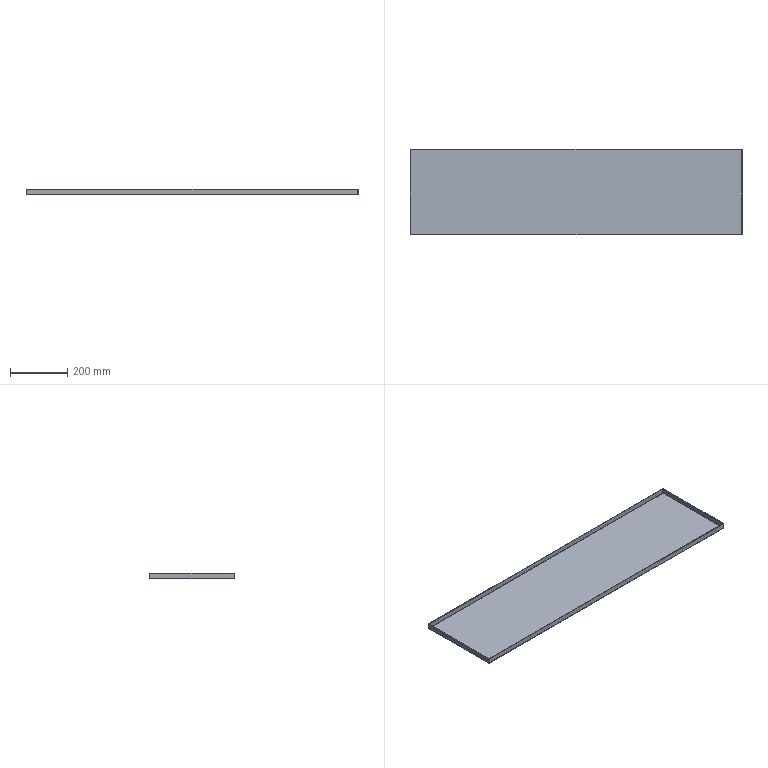Part | STEP file | Part 11 | 1 solid | 38 faces | box 1160 x 300 x 20 mm | volume 796554 mm3 | plane 22 | spline 8 | cylinder 8 | commonest cylinder face diameters 1 x4 5 x4
STEP:
#1=CARTESIAN_POINT('',(-577.5,-147.5,-2.));
#2=VERTEX_POINT('',#1);
#3=CARTESIAN_POINT('',(-577.5,147.5,-2.));
#4=VERTEX_POINT('',#3);
#5=CARTESIAN_POINT('',(-577.5,-147.5,-2.));
#6=DIRECTION('',(0.,1.,0.));
#7=VECTOR('',#6,1000.);
#8=LINE('',#5,#7);
#9=EDGE_CURVE('',#2,#4,#8,.T.);
#10=ORIENTED_EDGE('',*,*,#9,.T.);
#11=CARTESIAN_POINT('',(577.5,147.5,-2.));
#12=VERTEX_POINT('',#11);
#13=CARTESIAN_POINT('',(-577.5,147.5,-2.));
#14=DIRECTION('',(1.,0.,0.));
#15=VECTOR('',#14,1000.);
#16=LINE('',#13,#15);
#17=EDGE_CURVE('',#4,#12,#16,.T.);
#18=ORIENTED_EDGE('',*,*,#17,.T.);
#19=CARTESIAN_POINT('',(577.5,-147.5,-2.));
#20=VERTEX_POINT('',#19);
#21=CARTESIAN_POINT('',(577.5,147.5,-2.));
#22=DIRECTION('',(0.,-1.,0.));
#23=VECTOR('',#22,1000.);
#24=LINE('',#21,#23);
#25=EDGE_CURVE('',#12,#20,#24,.T.);
#26=ORIENTED_EDGE('',*,*,#25,.T.);
#27=CARTESIAN_POINT('',(577.5,-147.5,-2.));
#28=DIRECTION('',(-1.,0.,0.));
#29=VECTOR('',#28,1000.);
#30=LINE('',#27,#29);
#31=EDGE_CURVE('',#20,#2,#30,.T.);
#32=ORIENTED_EDGE('',*,*,#31,.T.);
#33=EDGE_LOOP('',(#10,#18,#26,#32));
#34=FACE_OUTER_BOUND('',#33,.T.);
#35=CARTESIAN_POINT('',(0.,0.,-2.));
#36=DIRECTION('',(0.,0.,1.));
#37=DIRECTION('',(1.,0.,0.));
#38=AXIS2_PLACEMENT_3D('',#35,#36,#37);
#39=PLANE('',#38);
#40=ADVANCED_FACE('',(#34),#39,.F.);
#41=CARTESIAN_POINT('',(-577.5,147.5,0.));
#42=VERTEX_POINT('',#41);
#43=CARTESIAN_POINT('',(577.5,147.5,0.));
#44=VERTEX_POINT('',#43);
#45=CARTESIAN_POINT('',(-577.5,147.5,0.));
#46=DIRECTION('',(1.,0.,0.));
#47=VECTOR('',#46,1000.);
#48=LINE('',#45,#47);
#49=EDGE_CURVE('',#42,#44,#48,.T.);
#50=ORIENTED_EDGE('',*,*,#49,.F.);
#51=CARTESIAN_POINT('',(-577.5,-147.5,0.));
#52=VERTEX_POINT('',#51);
#53=CARTESIAN_POINT('',(-577.5,-147.5,0.));
#54=DIRECTION('',(0.,1.,0.));
#55=VECTOR('',#54,1000.);
#56=LINE('',#53,#55);
#57=EDGE_CURVE('',#52,#42,#56,.T.);
#58=ORIENTED_EDGE('',*,*,#57,.F.);
#59=CARTESIAN_POINT('',(577.5,-147.5,0.));
#60=VERTEX_POINT('',#59);
#61=CARTESIAN_POINT('',(577.5,-147.5,0.));
#62=DIRECTION('',(-1.,0.,0.));
#63=VECTOR('',#62,1000.);
#64=LINE('',#61,#63);
#65=EDGE_CURVE('',#60,#52,#64,.T.);
#66=ORIENTED_EDGE('',*,*,#65,.F.);
#67=CARTESIAN_POINT('',(577.5,147.5,0.));
#68=DIRECTION('',(0.,-1.,0.));
#69=VECTOR('',#68,1000.);
#70=LINE('',#67,#69);
#71=EDGE_CURVE('',#44,#60,#70,.T.);
#72=ORIENTED_EDGE('',*,*,#71,.F.);
#73=EDGE_LOOP('',(#50,#58,#66,#72));
#74=FACE_OUTER_BOUND('',#73,.T.);
#75=CARTESIAN_POINT('',(0.,0.,0.));
#76=DIRECTION('',(0.,0.,1.));
#77=DIRECTION('',(1.,0.,0.));
#78=AXIS2_PLACEMENT_3D('',#75,#76,#77);
#79=PLANE('',#78);
#80=ADVANCED_FACE('',(#74),#79,.T.);
#81=CARTESIAN_POINT('',(577.293,150.,0.5));
#82=VERTEX_POINT('',#81);
#83=CARTESIAN_POINT('',(577.293,148.,0.5));
#84=VERTEX_POINT('',#83);
#85=CARTESIAN_POINT('',(577.293,148.,0.5));
#86=DIRECTION('',(0.,-1.,0.));
#87=VECTOR('',#86,1000.);
#88=LINE('',#85,#87);
#89=EDGE_CURVE('',#82,#84,#88,.T.);
#90=ORIENTED_EDGE('',*,*,#89,.T.);
#91=CARTESIAN_POINT('',(577.5,147.5,0.));
#92=CARTESIAN_POINT('',(577.465,147.631,0.));
#93=CARTESIAN_POINT('',(577.431,147.761,0.05389));
#94=CARTESIAN_POINT('',(577.362,147.946,0.239));
#95=CARTESIAN_POINT('',(577.327,148.,0.3691));
#96=CARTESIAN_POINT('',(577.293,148.,0.5));
#97=B_SPLINE_CURVE_WITH_KNOTS('',3,(#91,#92,#93,#94,#95,#96),.UNSPECIFIED.,.F.,.F.,(4,2,4),(0.,0.5,1.),.UNSPECIFIED.);
#98=EDGE_CURVE('',#44,#84,#97,.T.);
#99=ORIENTED_EDGE('',*,*,#98,.F.);
#100=CARTESIAN_POINT('',(577.5,147.5,0.));
#101=DIRECTION('',(0.,0.,-1.));
#102=VECTOR('',#101,1000.);
#103=LINE('',#100,#102);
#104=EDGE_CURVE('',#44,#12,#103,.T.);
#105=ORIENTED_EDGE('',*,*,#104,.T.);
#106=CARTESIAN_POINT('',(577.5,147.5,-2.));
#107=CARTESIAN_POINT('',(577.483,147.827,-2.));
#108=CARTESIAN_POINT('',(577.465,148.154,-1.935));
#109=CARTESIAN_POINT('',(577.431,148.759,-1.684));
#110=CARTESIAN_POINT('',(577.414,149.036,-1.499));
#111=CARTESIAN_POINT('',(577.379,149.499,-1.036));
#112=CARTESIAN_POINT('',(577.362,149.684,-0.759));
#113=CARTESIAN_POINT('',(577.327,149.935,-0.1544));
#114=CARTESIAN_POINT('',(577.31,150.,0.1728));
#115=CARTESIAN_POINT('',(577.293,150.,0.5));
#116=B_SPLINE_CURVE_WITH_KNOTS('',3,(#106,#107,#108,#109,#110,#111,#112,#113,#114,#115),.UNSPECIFIED.,.F.,.F.,(4,2,2,2,4),(0.,0.25,0.5,0.75,1.),.UNSPECIFIED.);
#117=EDGE_CURVE('',#12,#82,#116,.T.);
#118=ORIENTED_EDGE('',*,*,#117,.T.);
#119=EDGE_LOOP('',(#90,#99,#105,#118));
#120=FACE_OUTER_BOUND('',#119,.T.);
#121=CARTESIAN_POINT('',(577.5,147.5,-2.02));
#122=CARTESIAN_POINT('',(577.483,147.83,-2.02));
#123=CARTESIAN_POINT('',(577.465,148.16,-1.954));
#124=CARTESIAN_POINT('',(577.431,148.769,-1.702));
#125=CARTESIAN_POINT('',(577.414,149.049,-1.515));
#126=CARTESIAN_POINT('',(577.379,149.515,-1.049));
#127=CARTESIAN_POINT('',(577.362,149.702,-0.7691));
#128=CARTESIAN_POINT('',(577.327,149.954,-0.1596));
#129=CARTESIAN_POINT('',(577.31,150.02,0.1701));
#130=CARTESIAN_POINT('',(577.293,150.02,0.5));
#131=CARTESIAN_POINT('',(577.5,147.5,-2.));
#132=CARTESIAN_POINT('',(577.483,147.827,-2.));
#133=CARTESIAN_POINT('',(577.465,148.154,-1.935));
#134=CARTESIAN_POINT('',(577.431,148.759,-1.684));
#135=CARTESIAN_POINT('',(577.414,149.036,-1.499));
#136=CARTESIAN_POINT('',(577.379,149.499,-1.036));
#137=CARTESIAN_POINT('',(577.362,149.684,-0.759));
#138=CARTESIAN_POINT('',(577.327,149.935,-0.1544));
#139=CARTESIAN_POINT('',(577.31,150.,0.1727));
#140=CARTESIAN_POINT('',(577.293,150.,0.5));
#141=CARTESIAN_POINT('',(577.5,147.5,0.));
#142=CARTESIAN_POINT('',(577.483,147.565,0.));
#143=CARTESIAN_POINT('',(577.465,147.631,0.01301));
#144=CARTESIAN_POINT('',(577.431,147.752,0.06311));
#145=CARTESIAN_POINT('',(577.414,147.807,0.1002));
#146=CARTESIAN_POINT('',(577.379,147.9,0.1927));
#147=CARTESIAN_POINT('',(577.362,147.937,0.2482));
#148=CARTESIAN_POINT('',(577.327,147.987,0.3691));
#149=CARTESIAN_POINT('',(577.31,148.,0.4345));
#150=CARTESIAN_POINT('',(577.293,148.,0.5));
#151=CARTESIAN_POINT('',(577.5,147.5,0.0202));
#152=CARTESIAN_POINT('',(577.483,147.563,0.0202));
#153=CARTESIAN_POINT('',(577.465,147.626,0.03269));
#154=CARTESIAN_POINT('',(577.431,147.742,0.08076));
#155=CARTESIAN_POINT('',(577.414,147.795,0.1163));
#156=CARTESIAN_POINT('',(577.379,147.884,0.2051));
#157=CARTESIAN_POINT('',(577.362,147.919,0.2584));
#158=CARTESIAN_POINT('',(577.327,147.967,0.3744));
#159=CARTESIAN_POINT('',(577.31,147.98,0.4372));
#160=CARTESIAN_POINT('',(577.293,147.98,0.5));
#161=B_SPLINE_SURFACE_WITH_KNOTS('',1,3,((#121,#122,#123,#124,#125,#126,#127,#128,#129,#130),(#131,#132,#133,#134,#135,#136,#137,#138,#139,#140),(#141,#142,#143,#144,#145,#146,#147,#148,#149,#150),(#151,#152,#153,#154,#155,#156,#157,#158,#159,#160)),.UNSPECIFIED.,.F.,.F.,.F.,(2,1,1,2),(4,2,2,2,4),(-0.01,0.,1.,1.01),(0.,0.25,0.5,0.75,1.),.UNSPECIFIED.);
#162=ADVANCED_FACE('',(#120),#161,.F.);
#163=CARTESIAN_POINT('',(-577.293,148.,0.5));
#164=VERTEX_POINT('',#163);
#165=CARTESIAN_POINT('',(-577.293,148.,0.5));
#166=CARTESIAN_POINT('',(-577.327,148.,0.3691));
#167=CARTESIAN_POINT('',(-577.362,147.946,0.239));
#168=CARTESIAN_POINT('',(-577.431,147.761,0.05389));
#169=CARTESIAN_POINT('',(-577.465,147.631,0.));
#170=CARTESIAN_POINT('',(-577.5,147.5,0.));
#171=B_SPLINE_CURVE_WITH_KNOTS('',3,(#165,#166,#167,#168,#169,#170),.UNSPECIFIED.,.F.,.F.,(4,2,4),(0.,0.5,1.),.UNSPECIFIED.);
#172=EDGE_CURVE('',#164,#42,#171,.T.);
#173=ORIENTED_EDGE('',*,*,#172,.F.);
#174=CARTESIAN_POINT('',(-577.293,150.,0.5));
#175=VERTEX_POINT('',#174);
#176=CARTESIAN_POINT('',(-577.293,148.,0.5));
#177=DIRECTION('',(0.,-1.,0.));
#178=VECTOR('',#177,1000.);
#179=LINE('',#176,#178);
#180=EDGE_CURVE('',#175,#164,#179,.T.);
#181=ORIENTED_EDGE('',*,*,#180,.F.);
#182=CARTESIAN_POINT('',(-577.293,150.,0.5));
#183=CARTESIAN_POINT('',(-577.31,150.,0.1728));
#184=CARTESIAN_POINT('',(-577.327,149.935,-0.1544));
#185=CARTESIAN_POINT('',(-577.362,149.684,-0.759));
#186=CARTESIAN_POINT('',(-577.379,149.499,-1.036));
#187=CARTESIAN_POINT('',(-577.414,149.036,-1.499));
#188=CARTESIAN_POINT('',(-577.431,148.759,-1.684));
#189=CARTESIAN_POINT('',(-577.465,148.154,-1.935));
#190=CARTESIAN_POINT('',(-577.483,147.827,-2.));
#191=CARTESIAN_POINT('',(-577.5,147.5,-2.));
#192=B_SPLINE_CURVE_WITH_KNOTS('',3,(#182,#183,#184,#185,#186,#187,#188,#189,#190,#191),.UNSPECIFIED.,.F.,.F.,(4,2,2,2,4),(0.,0.25,0.5,0.75,1.),.UNSPECIFIED.);
#193=EDGE_CURVE('',#175,#4,#192,.T.);
#194=ORIENTED_EDGE('',*,*,#193,.T.);
#195=CARTESIAN_POINT('',(-577.5,147.5,0.));
#196=DIRECTION('',(0.,0.,-1.));
#197=VECTOR('',#196,1000.);
#198=LINE('',#195,#197);
#199=EDGE_CURVE('',#42,#4,#198,.T.);
#200=ORIENTED_EDGE('',*,*,#199,.F.);
#201=EDGE_LOOP('',(#173,#181,#194,#200));
#202=FACE_OUTER_BOUND('',#201,.T.);
#203=CARTESIAN_POINT('',(-577.293,150.02,0.5));
#204=CARTESIAN_POINT('',(-577.31,150.02,0.1701));
#205=CARTESIAN_POINT('',(-577.327,149.954,-0.1596));
#206=CARTESIAN_POINT('',(-577.362,149.702,-0.7691));
#207=CARTESIAN_POINT('',(-577.379,149.515,-1.049));
#208=CARTESIAN_POINT('',(-577.414,149.049,-1.515));
#209=CARTESIAN_POINT('',(-577.431,148.769,-1.702));
#210=CARTESIAN_POINT('',(-577.465,148.16,-1.954));
#211=CARTESIAN_POINT('',(-577.483,147.83,-2.02));
#212=CARTESIAN_POINT('',(-577.5,147.5,-2.02));
#213=CARTESIAN_POINT('',(-577.293,150.,0.5));
#214=CARTESIAN_POINT('',(-577.31,150.,0.1727));
#215=CARTESIAN_POINT('',(-577.327,149.935,-0.1544));
#216=CARTESIAN_POINT('',(-577.362,149.684,-0.759));
#217=CARTESIAN_POINT('',(-577.379,149.499,-1.036));
#218=CARTESIAN_POINT('',(-577.414,149.036,-1.499));
#219=CARTESIAN_POINT('',(-577.431,148.759,-1.684));
#220=CARTESIAN_POINT('',(-577.465,148.154,-1.935));
#221=CARTESIAN_POINT('',(-577.483,147.827,-2.));
#222=CARTESIAN_POINT('',(-577.5,147.5,-2.));
#223=CARTESIAN_POINT('',(-577.293,148.,0.5));
#224=CARTESIAN_POINT('',(-577.31,148.,0.4345));
#225=CARTESIAN_POINT('',(-577.327,147.987,0.3691));
#226=CARTESIAN_POINT('',(-577.362,147.937,0.2482));
#227=CARTESIAN_POINT('',(-577.379,147.9,0.1927));
#228=CARTESIAN_POINT('',(-577.414,147.807,0.1002));
#229=CARTESIAN_POINT('',(-577.431,147.752,0.06311));
#230=CARTESIAN_POINT('',(-577.465,147.631,0.01301));
#231=CARTESIAN_POINT('',(-577.483,147.565,0.));
#232=CARTESIAN_POINT('',(-577.5,147.5,0.));
#233=CARTESIAN_POINT('',(-577.293,147.98,0.5));
#234=CARTESIAN_POINT('',(-577.31,147.98,0.4372));
#235=CARTESIAN_POINT('',(-577.327,147.967,0.3744));
#236=CARTESIAN_POINT('',(-577.362,147.919,0.2584));
#237=CARTESIAN_POINT('',(-577.379,147.884,0.2051));
#238=CARTESIAN_POINT('',(-577.414,147.795,0.1163));
#239=CARTESIAN_POINT('',(-577.431,147.742,0.08076));
#240=CARTESIAN_POINT('',(-577.465,147.626,0.03269));
#241=CARTESIAN_POINT('',(-577.483,147.563,0.0202));
#242=CARTESIAN_POINT('',(-577.5,147.5,0.0202));
#243=B_SPLINE_SURFACE_WITH_KNOTS('',1,3,((#203,#204,#205,#206,#207,#208,#209,#210,#211,#212),(#213,#214,#215,#216,#217,#218,#219,#220,#221,#222),(#223,#224,#225,#226,#227,#228,#229,#230,#231,#232),(#233,#234,#235,#236,#237,#238,#239,#240,#241,#242)),.UNSPECIFIED.,.F.,.F.,.F.,(2,1,1,2),(4,2,2,2,4),(-0.01,0.,1.,1.01),(0.,0.25,0.5,0.75,1.),.UNSPECIFIED.);
#244=ADVANCED_FACE('',(#202),#243,.F.);
#245=ORIENTED_EDGE('',*,*,#17,.F.);
#246=ORIENTED_EDGE('',*,*,#193,.F.);
#247=CARTESIAN_POINT('',(0.,150.,0.5));
#248=DIRECTION('',(-1.,0.,0.));
#249=VECTOR('',#248,1000.);
#250=LINE('',#247,#249);
#251=EDGE_CURVE('',#82,#175,#250,.T.);
#252=ORIENTED_EDGE('',*,*,#251,.F.);
#253=ORIENTED_EDGE('',*,*,#117,.F.);
#254=EDGE_LOOP('',(#245,#246,#252,#253));
#255=FACE_OUTER_BOUND('',#254,.T.);
#256=CARTESIAN_POINT('',(-577.5,147.5,0.5));
#257=DIRECTION('',(-1.,0.,0.));
#258=DIRECTION('',(0.,1.,0.));
#259=AXIS2_PLACEMENT_3D('',#256,#257,#258);
#260=CYLINDRICAL_SURFACE('',#259,2.5);
#261=ADVANCED_FACE('',(#255),#260,.T.);
#262=ORIENTED_EDGE('',*,*,#49,.T.);
#263=ORIENTED_EDGE('',*,*,#98,.T.);
#264=CARTESIAN_POINT('',(580.,148.,0.5));
#265=DIRECTION('',(-1.,0.,0.));
#266=VECTOR('',#265,1000.);
#267=LINE('',#264,#266);
#268=EDGE_CURVE('',#84,#164,#267,.T.);
#269=ORIENTED_EDGE('',*,*,#268,.T.);
#270=ORIENTED_EDGE('',*,*,#172,.T.);
#271=EDGE_LOOP('',(#262,#263,#269,#270));
#272=FACE_OUTER_BOUND('',#271,.T.);
#273=CARTESIAN_POINT('',(-577.5,147.5,0.5));
#274=DIRECTION('',(-1.,0.,0.));
#275=DIRECTION('',(0.,1.,0.));
#276=AXIS2_PLACEMENT_3D('',#273,#274,#275);
#277=CYLINDRICAL_SURFACE('',#276,0.5);
#278=ADVANCED_FACE('',(#272),#277,.F.);
#279=CARTESIAN_POINT('',(577.293,148.,18.));
#280=VERTEX_POINT('',#279);
#281=CARTESIAN_POINT('',(577.293,150.,18.));
#282=VERTEX_POINT('',#281);
#283=CARTESIAN_POINT('',(577.293,150.,18.));
#284=DIRECTION('',(0.,1.,0.));
#285=VECTOR('',#284,1000.);
#286=LINE('',#283,#285);
#287=EDGE_CURVE('',#280,#282,#286,.T.);
#288=ORIENTED_EDGE('',*,*,#287,.F.);
#289=CARTESIAN_POINT('',(577.293,148.,0.));
#290=DIRECTION('',(0.,0.,1.));
#291=VECTOR('',#290,1000.);
#292=LINE('',#289,#291);
#293=EDGE_CURVE('',#84,#280,#292,.T.);
#294=ORIENTED_EDGE('',*,*,#293,.F.);
#295=ORIENTED_EDGE('',*,*,#89,.F.);
#296=CARTESIAN_POINT('',(577.293,150.,0.));
#297=DIRECTION('',(0.,0.,-1.));
#298=VECTOR('',#297,1000.);
#299=LINE('',#296,#298);
#300=EDGE_CURVE('',#282,#82,#299,.T.);
#301=ORIENTED_EDGE('',*,*,#300,.F.);
#302=EDGE_LOOP('',(#288,#294,#295,#301));
#303=FACE_OUTER_BOUND('',#302,.T.);
#304=CARTESIAN_POINT('',(577.293,148.,0.));
#305=DIRECTION('',(1.,0.,0.));
#306=DIRECTION('',(0.,0.,-1.));
#307=AXIS2_PLACEMENT_3D('',#304,#305,#306);
#308=PLANE('',#307);
#309=ADVANCED_FACE('',(#303),#308,.T.);
#310=CARTESIAN_POINT('',(-577.293,150.,18.));
#311=VERTEX_POINT('',#310);
#312=CARTESIAN_POINT('',(-577.293,150.,0.));
#313=DIRECTION('',(0.,0.,-1.));
#314=VECTOR('',#313,1000.);
#315=LINE('',#312,#314);
#316=EDGE_CURVE('',#311,#175,#315,.T.);
#317=ORIENTED_EDGE('',*,*,#316,.F.);
#318=CARTESIAN_POINT('',(-580.,150.,18.));
#319=DIRECTION('',(-1.,0.,0.));
#320=VECTOR('',#319,1000.);
#321=LINE('',#318,#320);
#322=EDGE_CURVE('',#282,#311,#321,.T.);
#323=ORIENTED_EDGE('',*,*,#322,.F.);
#324=ORIENTED_EDGE('',*,*,#300,.T.);
#325=ORIENTED_EDGE('',*,*,#251,.T.);
#326=EDGE_LOOP('',(#317,#323,#324,#325));
#327=FACE_OUTER_BOUND('',#326,.T.);
#328=CARTESIAN_POINT('',(0.,150.,0.));
#329=DIRECTION('',(0.,1.,0.));
#330=DIRECTION('',(0.,0.,1.));
#331=AXIS2_PLACEMENT_3D('',#328,#329,#330);
#332=PLANE('',#331);
#333=ADVANCED_FACE('',(#327),#332,.T.);
#334=CARTESIAN_POINT('',(-577.293,148.,18.));
#335=VERTEX_POINT('',#334);
#336=CARTESIAN_POINT('',(0.,148.,18.));
#337=DIRECTION('',(-1.,0.,0.));
#338=VECTOR('',#337,1000.);
#339=LINE('',#336,#338);
#340=EDGE_CURVE('',#280,#335,#339,.T.);
#341=ORIENTED_EDGE('',*,*,#340,.T.);
#342=CARTESIAN_POINT('',(-577.293,148.,0.));
#343=DIRECTION('',(0.,0.,1.));
#344=VECTOR('',#343,1000.);
#345=LINE('',#342,#344);
#346=EDGE_CURVE('',#164,#335,#345,.T.);
#347=ORIENTED_EDGE('',*,*,#346,.F.);
#348=ORIENTED_EDGE('',*,*,#268,.F.);
#349=ORIENTED_EDGE('',*,*,#293,.T.);
#350=EDGE_LOOP('',(#341,#347,#348,#349));
#351=FACE_OUTER_BOUND('',#350,.T.);
#352=CARTESIAN_POINT('',(0.,148.,0.));
#353=DIRECTION('',(0.,1.,0.));
#354=DIRECTION('',(0.,0.,1.));
#355=AXIS2_PLACEMENT_3D('',#352,#353,#354);
#356=PLANE('',#355);
#357=ADVANCED_FACE('',(#351),#356,.F.);
#358=CARTESIAN_POINT('',(-577.293,148.,18.));
#359=DIRECTION('',(0.,1.,0.));
#360=VECTOR('',#359,1000.);
#361=LINE('',#358,#360);
#362=EDGE_CURVE('',#335,#311,#361,.T.);
#363=ORIENTED_EDGE('',*,*,#362,.F.);
#364=ORIENTED_EDGE('',*,*,#340,.F.);
#365=ORIENTED_EDGE('',*,*,#287,.T.);
#366=ORIENTED_EDGE('',*,*,#322,.T.);
#367=EDGE_LOOP('',(#363,#364,#365,#366));
#368=FACE_OUTER_BOUND('',#367,.T.);
#369=CARTESIAN_POINT('',(-580.,150.,18.));
#370=DIRECTION('',(0.,0.,1.));
#371=DIRECTION('',(0.,-1.,0.));
#372=AXIS2_PLACEMENT_3D('',#369,#370,#371);
#373=PLANE('',#372);
#374=ADVANCED_FACE('',(#368),#373,.T.);
#375=ORIENTED_EDGE('',*,*,#346,.T.);
#376=ORIENTED_EDGE('',*,*,#362,.T.);
#377=ORIENTED_EDGE('',*,*,#316,.T.);
#378=ORIENTED_EDGE('',*,*,#180,.T.);
#379=EDGE_LOOP('',(#375,#376,#377,#378));
#380=FACE_OUTER_BOUND('',#379,.T.);
#381=CARTESIAN_POINT('',(-577.293,148.,0.));
#382=DIRECTION('',(1.,0.,0.));
#383=DIRECTION('',(0.,0.,-1.));
#384=AXIS2_PLACEMENT_3D('',#381,#382,#383);
#385=PLANE('',#384);
#386=ADVANCED_FACE('',(#380),#385,.F.);
#387=CARTESIAN_POINT('',(580.,-147.293,0.5));
#388=VERTEX_POINT('',#387);
#389=CARTESIAN_POINT('',(578.,-147.293,0.5));
#390=VERTEX_POINT('',#389);
#391=CARTESIAN_POINT('',(578.,-147.293,0.5));
#392=DIRECTION('',(-1.,0.,0.));
#393=VECTOR('',#392,1000.);
#394=LINE('',#391,#393);
#395=EDGE_CURVE('',#388,#390,#394,.T.);
#396=ORIENTED_EDGE('',*,*,#395,.T.);
#397=CARTESIAN_POINT('',(577.5,-147.5,0.));
#398=CARTESIAN_POINT('',(577.631,-147.465,0.));
#399=CARTESIAN_POINT('',(577.761,-147.431,0.05389));
#400=CARTESIAN_POINT('',(577.946,-147.362,0.239));
#401=CARTESIAN_POINT('',(578.,-147.327,0.3691));
#402=CARTESIAN_POINT('',(578.,-147.293,0.5));
#403=B_SPLINE_CURVE_WITH_KNOTS('',3,(#397,#398,#399,#400,#401,#402),.UNSPECIFIED.,.F.,.F.,(4,2,4),(0.,0.5,1.),.UNSPECIFIED.);
#404=EDGE_CURVE('',#60,#390,#403,.T.);
#405=ORIENTED_EDGE('',*,*,#404,.F.);
#406=CARTESIAN_POINT('',(577.5,-147.5,0.));
#407=DIRECTION('',(0.,0.,-1.));
#408=VECTOR('',#407,1000.);
#409=LINE('',#406,#408);
#410=EDGE_CURVE('',#60,#20,#409,.T.);
#411=ORIENTED_EDGE('',*,*,#410,.T.);
#412=CARTESIAN_POINT('',(577.5,-147.5,-2.));
#413=CARTESIAN_POINT('',(577.827,-147.483,-2.));
#414=CARTESIAN_POINT('',(578.154,-147.465,-1.935));
#415=CARTESIAN_POINT('',(578.759,-147.431,-1.684));
#416=CARTESIAN_POINT('',(579.036,-147.414,-1.499));
#417=CARTESIAN_POINT('',(579.499,-147.379,-1.036));
#418=CARTESIAN_POINT('',(579.684,-147.362,-0.759));
#419=CARTESIAN_POINT('',(579.935,-147.327,-0.1544));
#420=CARTESIAN_POINT('',(580.,-147.31,0.1728));
#421=CARTESIAN_POINT('',(580.,-147.293,0.5));
#422=B_SPLINE_CURVE_WITH_KNOTS('',3,(#412,#413,#414,#415,#416,#417,#418,#419,#420,#421),.UNSPECIFIED.,.F.,.F.,(4,2,2,2,4),(0.,0.25,0.5,0.75,1.),.UNSPECIFIED.);
#423=EDGE_CURVE('',#20,#388,#422,.T.);
#424=ORIENTED_EDGE('',*,*,#423,.T.);
#425=EDGE_LOOP('',(#396,#405,#411,#424));
#426=FACE_OUTER_BOUND('',#425,.T.);
#427=CARTESIAN_POINT('',(577.5,-147.5,-2.02));
#428=CARTESIAN_POINT('',(577.83,-147.483,-2.02));
#429=CARTESIAN_POINT('',(578.16,-147.465,-1.954));
#430=CARTESIAN_POINT('',(578.769,-147.431,-1.702));
#431=CARTESIAN_POINT('',(579.049,-147.414,-1.515));
#432=CARTESIAN_POINT('',(579.515,-147.379,-1.049));
#433=CARTESIAN_POINT('',(579.702,-147.362,-0.7691));
#434=CARTESIAN_POINT('',(579.954,-147.327,-0.1596));
#435=CARTESIAN_POINT('',(580.02,-147.31,0.1701));
#436=CARTESIAN_POINT('',(580.02,-147.293,0.5));
#437=CARTESIAN_POINT('',(577.5,-147.5,-2.));
#438=CARTESIAN_POINT('',(577.827,-147.483,-2.));
#439=CARTESIAN_POINT('',(578.154,-147.465,-1.935));
#440=CARTESIAN_POINT('',(578.759,-147.431,-1.684));
#441=CARTESIAN_POINT('',(579.036,-147.414,-1.499));
#442=CARTESIAN_POINT('',(579.499,-147.379,-1.036));
#443=CARTESIAN_POINT('',(579.684,-147.362,-0.759));
#444=CARTESIAN_POINT('',(579.935,-147.327,-0.1544));
#445=CARTESIAN_POINT('',(580.,-147.31,0.1727));
#446=CARTESIAN_POINT('',(580.,-147.293,0.5));
#447=CARTESIAN_POINT('',(577.5,-147.5,0.));
#448=CARTESIAN_POINT('',(577.565,-147.483,0.));
#449=CARTESIAN_POINT('',(577.631,-147.465,0.01301));
#450=CARTESIAN_POINT('',(577.752,-147.431,0.06311));
#451=CARTESIAN_POINT('',(577.807,-147.414,0.1002));
#452=CARTESIAN_POINT('',(577.9,-147.379,0.1927));
#453=CARTESIAN_POINT('',(577.937,-147.362,0.2482));
#454=CARTESIAN_POINT('',(577.987,-147.327,0.3691));
#455=CARTESIAN_POINT('',(578.,-147.31,0.4345));
#456=CARTESIAN_POINT('',(578.,-147.293,0.5));
#457=CARTESIAN_POINT('',(577.5,-147.5,0.0202));
#458=CARTESIAN_POINT('',(577.563,-147.483,0.0202));
#459=CARTESIAN_POINT('',(577.626,-147.465,0.03269));
#460=CARTESIAN_POINT('',(577.742,-147.431,0.08076));
#461=CARTESIAN_POINT('',(577.795,-147.414,0.1163));
#462=CARTESIAN_POINT('',(577.884,-147.379,0.2051));
#463=CARTESIAN_POINT('',(577.919,-147.362,0.2584));
#464=CARTESIAN_POINT('',(577.967,-147.327,0.3744));
#465=CARTESIAN_POINT('',(577.98,-147.31,0.4372));
#466=CARTESIAN_POINT('',(577.98,-147.293,0.5));
#467=B_SPLINE_SURFACE_WITH_KNOTS('',1,3,((#427,#428,#429,#430,#431,#432,#433,#434,#435,#436),(#437,#438,#439,#440,#441,#442,#443,#444,#445,#446),(#447,#448,#449,#450,#451,#452,#453,#454,#455,#456),(#457,#458,#459,#460,#461,#462,#463,#464,#465,#466)),.UNSPECIFIED.,.F.,.F.,.F.,(2,1,1,2),(4,2,2,2,4),(-0.01,0.,1.,1.01),(0.,0.25,0.5,0.75,1.),.UNSPECIFIED.);
#468=ADVANCED_FACE('',(#426),#467,.F.);
#469=CARTESIAN_POINT('',(578.,147.293,0.5));
#470=VERTEX_POINT('',#469);
#471=CARTESIAN_POINT('',(578.,147.293,0.5));
#472=CARTESIAN_POINT('',(578.,147.327,0.3691));
#473=CARTESIAN_POINT('',(577.946,147.362,0.239));
#474=CARTESIAN_POINT('',(577.761,147.431,0.05389));
#475=CARTESIAN_POINT('',(577.631,147.465,0.));
#476=CARTESIAN_POINT('',(577.5,147.5,0.));
#477=B_SPLINE_CURVE_WITH_KNOTS('',3,(#471,#472,#473,#474,#475,#476),.UNSPECIFIED.,.F.,.F.,(4,2,4),(0.,0.5,1.),.UNSPECIFIED.);
#478=EDGE_CURVE('',#470,#44,#477,.T.);
#479=ORIENTED_EDGE('',*,*,#478,.F.);
#480=CARTESIAN_POINT('',(580.,147.293,0.5));
#481=VERTEX_POINT('',#480);
#482=CARTESIAN_POINT('',(578.,147.293,0.5));
#483=DIRECTION('',(-1.,0.,0.));
#484=VECTOR('',#483,1000.);
#485=LINE('',#482,#484);
#486=EDGE_CURVE('',#481,#470,#485,.T.);
#487=ORIENTED_EDGE('',*,*,#486,.F.);
#488=CARTESIAN_POINT('',(580.,147.293,0.5));
#489=CARTESIAN_POINT('',(580.,147.31,0.1728));
#490=CARTESIAN_POINT('',(579.935,147.327,-0.1544));
#491=CARTESIAN_POINT('',(579.684,147.362,-0.759));
#492=CARTESIAN_POINT('',(579.499,147.379,-1.036));
#493=CARTESIAN_POINT('',(579.036,147.414,-1.499));
#494=CARTESIAN_POINT('',(578.759,147.431,-1.684));
#495=CARTESIAN_POINT('',(578.154,147.465,-1.935));
#496=CARTESIAN_POINT('',(577.827,147.483,-2.));
#497=CARTESIAN_POINT('',(577.5,147.5,-2.));
#498=B_SPLINE_CURVE_WITH_KNOTS('',3,(#488,#489,#490,#491,#492,#493,#494,#495,#496,#497),.UNSPECIFIED.,.F.,.F.,(4,2,2,2,4),(0.,0.25,0.5,0.75,1.),.UNSPECIFIED.);
#499=EDGE_CURVE('',#481,#12,#498,.T.);
#500=ORIENTED_EDGE('',*,*,#499,.T.);
#501=ORIENTED_EDGE('',*,*,#104,.F.);
#502=EDGE_LOOP('',(#479,#487,#500,#501));
#503=FACE_OUTER_BOUND('',#502,.T.);
#504=CARTESIAN_POINT('',(580.02,147.293,0.5));
#505=CARTESIAN_POINT('',(580.02,147.31,0.1701));
#506=CARTESIAN_POINT('',(579.954,147.327,-0.1596));
#507=CARTESIAN_POINT('',(579.702,147.362,-0.7691));
#508=CARTESIAN_POINT('',(579.515,147.379,-1.049));
#509=CARTESIAN_POINT('',(579.049,147.414,-1.515));
#510=CARTESIAN_POINT('',(578.769,147.431,-1.702));
#511=CARTESIAN_POINT('',(578.16,147.465,-1.954));
#512=CARTESIAN_POINT('',(577.83,147.483,-2.02));
#513=CARTESIAN_POINT('',(577.5,147.5,-2.02));
#514=CARTESIAN_POINT('',(580.,147.293,0.5));
#515=CARTESIAN_POINT('',(580.,147.31,0.1727));
#516=CARTESIAN_POINT('',(579.935,147.327,-0.1544));
#517=CARTESIAN_POINT('',(579.684,147.362,-0.759));
#518=CARTESIAN_POINT('',(579.499,147.379,-1.036));
#519=CARTESIAN_POINT('',(579.036,147.414,-1.499));
#520=CARTESIAN_POINT('',(578.759,147.431,-1.684));
#521=CARTESIAN_POINT('',(578.154,147.465,-1.935));
#522=CARTESIAN_POINT('',(577.827,147.483,-2.));
#523=CARTESIAN_POINT('',(577.5,147.5,-2.));
#524=CARTESIAN_POINT('',(578.,147.293,0.5));
#525=CARTESIAN_POINT('',(578.,147.31,0.4345));
#526=CARTESIAN_POINT('',(577.987,147.327,0.3691));
#527=CARTESIAN_POINT('',(577.937,147.362,0.2482));
#528=CARTESIAN_POINT('',(577.9,147.379,0.1927));
#529=CARTESIAN_POINT('',(577.807,147.414,0.1002));
#530=CARTESIAN_POINT('',(577.752,147.431,0.06311));
#531=CARTESIAN_POINT('',(577.631,147.465,0.01301));
#532=CARTESIAN_POINT('',(577.565,147.483,0.));
#533=CARTESIAN_POINT('',(577.5,147.5,0.));
#534=CARTESIAN_POINT('',(577.98,147.293,0.5));
#535=CARTESIAN_POINT('',(577.98,147.31,0.4372));
#536=CARTESIAN_POINT('',(577.967,147.327,0.3744));
#537=CARTESIAN_POINT('',(577.919,147.362,0.2584));
#538=CARTESIAN_POINT('',(577.884,147.379,0.2051));
#539=CARTESIAN_POINT('',(577.795,147.414,0.1163));
#540=CARTESIAN_POINT('',(577.742,147.431,0.08076));
#541=CARTESIAN_POINT('',(577.626,147.465,0.03269));
#542=CARTESIAN_POINT('',(577.563,147.483,0.0202));
#543=CARTESIAN_POINT('',(577.5,147.5,0.0202));
#544=B_SPLINE_SURFACE_WITH_KNOTS('',1,3,((#504,#505,#506,#507,#508,#509,#510,#511,#512,#513),(#514,#515,#516,#517,#518,#519,#520,#521,#522,#523),(#524,#525,#526,#527,#528,#529,#530,#531,#532,#533),(#534,#535,#536,#537,#538,#539,#540,#541,#542,#543)),.UNSPECIFIED.,.F.,.F.,.F.,(2,1,1,2),(4,2,2,2,4),(-0.01,0.,1.,1.01),(0.,0.25,0.5,0.75,1.),.UNSPECIFIED.);
#545=ADVANCED_FACE('',(#503),#544,.F.);
#546=ORIENTED_EDGE('',*,*,#25,.F.);
#547=ORIENTED_EDGE('',*,*,#499,.F.);
#548=CARTESIAN_POINT('',(580.,-150.,0.5));
#549=DIRECTION('',(0.,-1.,0.));
#550=VECTOR('',#549,1000.);
#551=LINE('',#548,#550);
#552=EDGE_CURVE('',#481,#388,#551,.T.);
#553=ORIENTED_EDGE('',*,*,#552,.T.);
#554=ORIENTED_EDGE('',*,*,#423,.F.);
#555=EDGE_LOOP('',(#546,#547,#553,#554));
#556=FACE_OUTER_BOUND('',#555,.T.);
#557=CARTESIAN_POINT('',(577.5,147.5,0.5));
#558=DIRECTION('',(0.,1.,0.));
#559=DIRECTION('',(1.,0.,0.));
#560=AXIS2_PLACEMENT_3D('',#557,#558,#559);
#561=CYLINDRICAL_SURFACE('',#560,2.5);
#562=ADVANCED_FACE('',(#556),#561,.T.);
#563=ORIENTED_EDGE('',*,*,#71,.T.);
#564=ORIENTED_EDGE('',*,*,#404,.T.);
#565=CARTESIAN_POINT('',(578.,-150.,0.5));
#566=DIRECTION('',(0.,1.,0.));
#567=VECTOR('',#566,1000.);
#568=LINE('',#565,#567);
#569=EDGE_CURVE('',#390,#470,#568,.T.);
#570=ORIENTED_EDGE('',*,*,#569,.T.);
#571=ORIENTED_EDGE('',*,*,#478,.T.);
#572=EDGE_LOOP('',(#563,#564,#570,#571));
#573=FACE_OUTER_BOUND('',#572,.T.);
#574=CARTESIAN_POINT('',(577.5,147.5,0.5));
#575=DIRECTION('',(0.,1.,0.));
#576=DIRECTION('',(1.,0.,0.));
#577=AXIS2_PLACEMENT_3D('',#574,#575,#576);
#578=CYLINDRICAL_SURFACE('',#577,0.5);
#579=ADVANCED_FACE('',(#573),#578,.F.);
#580=CARTESIAN_POINT('',(578.,-147.293,18.));
#581=VERTEX_POINT('',#580);
#582=CARTESIAN_POINT('',(580.,-147.293,18.));
#583=VERTEX_POINT('',#582);
#584=CARTESIAN_POINT('',(580.,-147.293,18.));
#585=DIRECTION('',(1.,0.,0.));
#586=VECTOR('',#585,1000.);
#587=LINE('',#584,#586);
#588=EDGE_CURVE('',#581,#583,#587,.T.);
#589=ORIENTED_EDGE('',*,*,#588,.F.);
#590=CARTESIAN_POINT('',(578.,-147.293,0.));
#591=DIRECTION('',(0.,0.,1.));
#592=VECTOR('',#591,1000.);
#593=LINE('',#590,#592);
#594=EDGE_CURVE('',#390,#581,#593,.T.);
#595=ORIENTED_EDGE('',*,*,#594,.F.);
#596=ORIENTED_EDGE('',*,*,#395,.F.);
#597=CARTESIAN_POINT('',(580.,-147.293,0.));
#598=DIRECTION('',(0.,0.,1.));
#599=VECTOR('',#598,1000.);
#600=LINE('',#597,#599);
#601=EDGE_CURVE('',#388,#583,#600,.T.);
#602=ORIENTED_EDGE('',*,*,#601,.T.);
#603=EDGE_LOOP('',(#589,#595,#596,#602));
#604=FACE_OUTER_BOUND('',#603,.T.);
#605=CARTESIAN_POINT('',(578.,-147.293,0.));
#606=DIRECTION('',(0.,-1.,0.));
#607=DIRECTION('',(0.,0.,-1.));
#608=AXIS2_PLACEMENT_3D('',#605,#606,#607);
#609=PLANE('',#608);
#610=ADVANCED_FACE('',(#604),#609,.T.);
#611=ORIENTED_EDGE('',*,*,#552,.F.);
#612=CARTESIAN_POINT('',(580.,147.293,18.));
#613=VERTEX_POINT('',#612);
#614=CARTESIAN_POINT('',(580.,147.293,0.));
#615=DIRECTION('',(0.,0.,1.));
#616=VECTOR('',#615,1000.);
#617=LINE('',#614,#616);
#618=EDGE_CURVE('',#481,#613,#617,.T.);
#619=ORIENTED_EDGE('',*,*,#618,.T.);
#620=CARTESIAN_POINT('',(580.,-150.,18.));
#621=DIRECTION('',(0.,1.,0.));
#622=VECTOR('',#621,1000.);
#623=LINE('',#620,#622);
#624=EDGE_CURVE('',#583,#613,#623,.T.);
#625=ORIENTED_EDGE('',*,*,#624,.F.);
#626=ORIENTED_EDGE('',*,*,#601,.F.);
#627=EDGE_LOOP('',(#611,#619,#625,#626));
#628=FACE_OUTER_BOUND('',#627,.T.);
#629=CARTESIAN_POINT('',(580.,0.,0.));
#630=DIRECTION('',(-1.,0.,0.));
#631=DIRECTION('',(0.,-1.,0.));
#632=AXIS2_PLACEMENT_3D('',#629,#630,#631);
#633=PLANE('',#632);
#634=ADVANCED_FACE('',(#628),#633,.F.);
#635=CARTESIAN_POINT('',(578.,147.293,18.));
#636=VERTEX_POINT('',#635);
#637=CARTESIAN_POINT('',(578.,147.293,0.));
#638=DIRECTION('',(0.,0.,1.));
#639=VECTOR('',#638,1000.);
#640=LINE('',#637,#639);
#641=EDGE_CURVE('',#470,#636,#640,.T.);
#642=ORIENTED_EDGE('',*,*,#641,.F.);
#643=ORIENTED_EDGE('',*,*,#569,.F.);
#644=ORIENTED_EDGE('',*,*,#594,.T.);
#645=CARTESIAN_POINT('',(578.,0.,18.));
#646=DIRECTION('',(0.,1.,0.));
#647=VECTOR('',#646,1000.);
#648=LINE('',#645,#647);
#649=EDGE_CURVE('',#581,#636,#648,.T.);
#650=ORIENTED_EDGE('',*,*,#649,.T.);
#651=EDGE_LOOP('',(#642,#643,#644,#650));
#652=FACE_OUTER_BOUND('',#651,.T.);
#653=CARTESIAN_POINT('',(578.,0.,0.));
#654=DIRECTION('',(-1.,0.,0.));
#655=DIRECTION('',(0.,-1.,0.));
#656=AXIS2_PLACEMENT_3D('',#653,#654,#655);
#657=PLANE('',#656);
#658=ADVANCED_FACE('',(#652),#657,.T.);
#659=CARTESIAN_POINT('',(578.,147.293,18.));
#660=DIRECTION('',(1.,0.,0.));
#661=VECTOR('',#660,1000.);
#662=LINE('',#659,#661);
#663=EDGE_CURVE('',#636,#613,#662,.T.);
#664=ORIENTED_EDGE('',*,*,#663,.F.);
#665=ORIENTED_EDGE('',*,*,#649,.F.);
#666=ORIENTED_EDGE('',*,*,#588,.T.);
#667=ORIENTED_EDGE('',*,*,#624,.T.);
#668=EDGE_LOOP('',(#664,#665,#666,#667));
#669=FACE_OUTER_BOUND('',#668,.T.);
#670=CARTESIAN_POINT('',(580.,-150.,18.));
#671=DIRECTION('',(0.,0.,1.));
#672=DIRECTION('',(1.,0.,0.));
#673=AXIS2_PLACEMENT_3D('',#670,#671,#672);
#674=PLANE('',#673);
#675=ADVANCED_FACE('',(#669),#674,.T.);
#676=ORIENTED_EDGE('',*,*,#641,.T.);
#677=ORIENTED_EDGE('',*,*,#663,.T.);
#678=ORIENTED_EDGE('',*,*,#618,.F.);
#679=ORIENTED_EDGE('',*,*,#486,.T.);
#680=EDGE_LOOP('',(#676,#677,#678,#679));
#681=FACE_OUTER_BOUND('',#680,.T.);
#682=CARTESIAN_POINT('',(578.,147.293,0.));
#683=DIRECTION('',(0.,-1.,0.));
#684=DIRECTION('',(0.,0.,-1.));
#685=AXIS2_PLACEMENT_3D('',#682,#683,#684);
#686=PLANE('',#685);
#687=ADVANCED_FACE('',(#681),#686,.F.);
#688=CARTESIAN_POINT('',(-577.293,-150.,0.5));
#689=VERTEX_POINT('',#688);
#690=CARTESIAN_POINT('',(-577.293,-148.,0.5));
#691=VERTEX_POINT('',#690);
#692=CARTESIAN_POINT('',(-577.293,-148.,0.5));
#693=DIRECTION('',(0.,1.,0.));
#694=VECTOR('',#693,1000.);
#695=LINE('',#692,#694);
#696=EDGE_CURVE('',#689,#691,#695,.T.);
#697=ORIENTED_EDGE('',*,*,#696,.T.);
#698=CARTESIAN_POINT('',(-577.5,-147.5,0.));
#699=CARTESIAN_POINT('',(-577.465,-147.631,0.));
#700=CARTESIAN_POINT('',(-577.431,-147.761,0.05389));
#701=CARTESIAN_POINT('',(-577.362,-147.946,0.239));
#702=CARTESIAN_POINT('',(-577.327,-148.,0.3691));
#703=CARTESIAN_POINT('',(-577.293,-148.,0.5));
#704=B_SPLINE_CURVE_WITH_KNOTS('',3,(#698,#699,#700,#701,#702,#703),.UNSPECIFIED.,.F.,.F.,(4,2,4),(0.,0.5,1.),.UNSPECIFIED.);
#705=EDGE_CURVE('',#52,#691,#704,.T.);
#706=ORIENTED_EDGE('',*,*,#705,.F.);
#707=CARTESIAN_POINT('',(-577.5,-147.5,0.));
#708=DIRECTION('',(0.,0.,-1.));
#709=VECTOR('',#708,1000.);
#710=LINE('',#707,#709);
#711=EDGE_CURVE('',#52,#2,#710,.T.);
#712=ORIENTED_EDGE('',*,*,#711,.T.);
#713=CARTESIAN_POINT('',(-577.5,-147.5,-2.));
#714=CARTESIAN_POINT('',(-577.483,-147.827,-2.));
#715=CARTESIAN_POINT('',(-577.465,-148.154,-1.935));
#716=CARTESIAN_POINT('',(-577.431,-148.759,-1.684));
#717=CARTESIAN_POINT('',(-577.414,-149.036,-1.499));
#718=CARTESIAN_POINT('',(-577.379,-149.499,-1.036));
#719=CARTESIAN_POINT('',(-577.362,-149.684,-0.759));
#720=CARTESIAN_POINT('',(-577.327,-149.935,-0.1544));
#721=CARTESIAN_POINT('',(-577.31,-150.,0.1728));
#722=CARTESIAN_POINT('',(-577.293,-150.,0.5));
#723=B_SPLINE_CURVE_WITH_KNOTS('',3,(#713,#714,#715,#716,#717,#718,#719,#720,#721,#722),.UNSPECIFIED.,.F.,.F.,(4,2,2,2,4),(0.,0.25,0.5,0.75,1.),.UNSPECIFIED.);
#724=EDGE_CURVE('',#2,#689,#723,.T.);
#725=ORIENTED_EDGE('',*,*,#724,.T.);
#726=EDGE_LOOP('',(#697,#706,#712,#725));
#727=FACE_OUTER_BOUND('',#726,.T.);
#728=CARTESIAN_POINT('',(-577.5,-147.5,-2.02));
#729=CARTESIAN_POINT('',(-577.483,-147.83,-2.02));
#730=CARTESIAN_POINT('',(-577.465,-148.16,-1.954));
#731=CARTESIAN_POINT('',(-577.431,-148.769,-1.702));
#732=CARTESIAN_POINT('',(-577.414,-149.049,-1.515));
#733=CARTESIAN_POINT('',(-577.379,-149.515,-1.049));
#734=CARTESIAN_POINT('',(-577.362,-149.702,-0.7691));
#735=CARTESIAN_POINT('',(-577.327,-149.954,-0.1596));
#736=CARTESIAN_POINT('',(-577.31,-150.02,0.1701));
#737=CARTESIAN_POINT('',(-577.293,-150.02,0.5));
#738=CARTESIAN_POINT('',(-577.5,-147.5,-2.));
#739=CARTESIAN_POINT('',(-577.483,-147.827,-2.));
#740=CARTESIAN_POINT('',(-577.465,-148.154,-1.935));
#741=CARTESIAN_POINT('',(-577.431,-148.759,-1.684));
#742=CARTESIAN_POINT('',(-577.414,-149.036,-1.499));
#743=CARTESIAN_POINT('',(-577.379,-149.499,-1.036));
#744=CARTESIAN_POINT('',(-577.362,-149.684,-0.759));
#745=CARTESIAN_POINT('',(-577.327,-149.935,-0.1544));
#746=CARTESIAN_POINT('',(-577.31,-150.,0.1727));
#747=CARTESIAN_POINT('',(-577.293,-150.,0.5));
#748=CARTESIAN_POINT('',(-577.5,-147.5,0.));
#749=CARTESIAN_POINT('',(-577.483,-147.565,0.));
#750=CARTESIAN_POINT('',(-577.465,-147.631,0.01301));
#751=CARTESIAN_POINT('',(-577.431,-147.752,0.06311));
#752=CARTESIAN_POINT('',(-577.414,-147.807,0.1002));
#753=CARTESIAN_POINT('',(-577.379,-147.9,0.1927));
#754=CARTESIAN_POINT('',(-577.362,-147.937,0.2482));
#755=CARTESIAN_POINT('',(-577.327,-147.987,0.3691));
#756=CARTESIAN_POINT('',(-577.31,-148.,0.4345));
#757=CARTESIAN_POINT('',(-577.293,-148.,0.5));
#758=CARTESIAN_POINT('',(-577.5,-147.5,0.0202));
#759=CARTESIAN_POINT('',(-577.483,-147.563,0.0202));
#760=CARTESIAN_POINT('',(-577.465,-147.626,0.03269));
#761=CARTESIAN_POINT('',(-577.431,-147.742,0.08076));
#762=CARTESIAN_POINT('',(-577.414,-147.795,0.1163));
#763=CARTESIAN_POINT('',(-577.379,-147.884,0.2051));
#764=CARTESIAN_POINT('',(-577.362,-147.919,0.2584));
#765=CARTESIAN_POINT('',(-577.327,-147.967,0.3744));
#766=CARTESIAN_POINT('',(-577.31,-147.98,0.4372));
#767=CARTESIAN_POINT('',(-577.293,-147.98,0.5));
#768=B_SPLINE_SURFACE_WITH_KNOTS('',1,3,((#728,#729,#730,#731,#732,#733,#734,#735,#736,#737),(#738,#739,#740,#741,#742,#743,#744,#745,#746,#747),(#748,#749,#750,#751,#752,#753,#754,#755,#756,#757),(#758,#759,#760,#761,#762,#763,#764,#765,#766,#767)),.UNSPECIFIED.,.F.,.F.,.F.,(2,1,1,2),(4,2,2,2,4),(-0.01,0.,1.,1.01),(0.,0.25,0.5,0.75,1.),.UNSPECIFIED.);
#769=ADVANCED_FACE('',(#727),#768,.F.);
#770=CARTESIAN_POINT('',(577.293,-148.,0.5));
#771=VERTEX_POINT('',#770);
#772=CARTESIAN_POINT('',(577.293,-148.,0.5));
#773=CARTESIAN_POINT('',(577.327,-148.,0.3691));
#774=CARTESIAN_POINT('',(577.362,-147.946,0.239));
#775=CARTESIAN_POINT('',(577.431,-147.761,0.05389));
#776=CARTESIAN_POINT('',(577.465,-147.631,0.));
#777=CARTESIAN_POINT('',(577.5,-147.5,0.));
#778=B_SPLINE_CURVE_WITH_KNOTS('',3,(#772,#773,#774,#775,#776,#777),.UNSPECIFIED.,.F.,.F.,(4,2,4),(0.,0.5,1.),.UNSPECIFIED.);
#779=EDGE_CURVE('',#771,#60,#778,.T.);
#780=ORIENTED_EDGE('',*,*,#779,.F.);
#781=CARTESIAN_POINT('',(577.293,-150.,0.5));
#782=VERTEX_POINT('',#781);
#783=CARTESIAN_POINT('',(577.293,-148.,0.5));
#784=DIRECTION('',(0.,1.,0.));
#785=VECTOR('',#784,1000.);
#786=LINE('',#783,#785);
#787=EDGE_CURVE('',#782,#771,#786,.T.);
#788=ORIENTED_EDGE('',*,*,#787,.F.);
#789=CARTESIAN_POINT('',(577.293,-150.,0.5));
#790=CARTESIAN_POINT('',(577.31,-150.,0.1728));
#791=CARTESIAN_POINT('',(577.327,-149.935,-0.1544));
#792=CARTESIAN_POINT('',(577.362,-149.684,-0.759));
#793=CARTESIAN_POINT('',(577.379,-149.499,-1.036));
#794=CARTESIAN_POINT('',(577.414,-149.036,-1.499));
#795=CARTESIAN_POINT('',(577.431,-148.759,-1.684));
#796=CARTESIAN_POINT('',(577.465,-148.154,-1.935));
#797=CARTESIAN_POINT('',(577.483,-147.827,-2.));
#798=CARTESIAN_POINT('',(577.5,-147.5,-2.));
#799=B_SPLINE_CURVE_WITH_KNOTS('',3,(#789,#790,#791,#792,#793,#794,#795,#796,#797,#798),.UNSPECIFIED.,.F.,.F.,(4,2,2,2,4),(0.,0.25,0.5,0.75,1.),.UNSPECIFIED.);
#800=EDGE_CURVE('',#782,#20,#799,.T.);
#801=ORIENTED_EDGE('',*,*,#800,.T.);
#802=ORIENTED_EDGE('',*,*,#410,.F.);
#803=EDGE_LOOP('',(#780,#788,#801,#802));
#804=FACE_OUTER_BOUND('',#803,.T.);
#805=CARTESIAN_POINT('',(577.293,-150.02,0.5));
#806=CARTESIAN_POINT('',(577.31,-150.02,0.1701));
#807=CARTESIAN_POINT('',(577.327,-149.954,-0.1596));
#808=CARTESIAN_POINT('',(577.362,-149.702,-0.7691));
#809=CARTESIAN_POINT('',(577.379,-149.515,-1.049));
#810=CARTESIAN_POINT('',(577.414,-149.049,-1.515));
#811=CARTESIAN_POINT('',(577.431,-148.769,-1.702));
#812=CARTESIAN_POINT('',(577.465,-148.16,-1.954));
#813=CARTESIAN_POINT('',(577.483,-147.83,-2.02));
#814=CARTESIAN_POINT('',(577.5,-147.5,-2.02));
#815=CARTESIAN_POINT('',(577.293,-150.,0.5));
#816=CARTESIAN_POINT('',(577.31,-150.,0.1727));
#817=CARTESIAN_POINT('',(577.327,-149.935,-0.1544));
#818=CARTESIAN_POINT('',(577.362,-149.684,-0.759));
#819=CARTESIAN_POINT('',(577.379,-149.499,-1.036));
#820=CARTESIAN_POINT('',(577.414,-149.036,-1.499));
#821=CARTESIAN_POINT('',(577.431,-148.759,-1.684));
#822=CARTESIAN_POINT('',(577.465,-148.154,-1.935));
#823=CARTESIAN_POINT('',(577.483,-147.827,-2.));
#824=CARTESIAN_POINT('',(577.5,-147.5,-2.));
#825=CARTESIAN_POINT('',(577.293,-148.,0.5));
#826=CARTESIAN_POINT('',(577.31,-148.,0.4345));
#827=CARTESIAN_POINT('',(577.327,-147.987,0.3691));
#828=CARTESIAN_POINT('',(577.362,-147.937,0.2482));
#829=CARTESIAN_POINT('',(577.379,-147.9,0.1927));
#830=CARTESIAN_POINT('',(577.414,-147.807,0.1002));
#831=CARTESIAN_POINT('',(577.431,-147.752,0.06311));
#832=CARTESIAN_POINT('',(577.465,-147.631,0.01301));
#833=CARTESIAN_POINT('',(577.483,-147.565,0.));
#834=CARTESIAN_POINT('',(577.5,-147.5,0.));
#835=CARTESIAN_POINT('',(577.293,-147.98,0.5));
#836=CARTESIAN_POINT('',(577.31,-147.98,0.4372));
#837=CARTESIAN_POINT('',(577.327,-147.967,0.3744));
#838=CARTESIAN_POINT('',(577.362,-147.919,0.2584));
#839=CARTESIAN_POINT('',(577.379,-147.884,0.2051));
#840=CARTESIAN_POINT('',(577.414,-147.795,0.1163));
#841=CARTESIAN_POINT('',(577.431,-147.742,0.08076));
#842=CARTESIAN_POINT('',(577.465,-147.626,0.03269));
#843=CARTESIAN_POINT('',(577.483,-147.563,0.0202));
#844=CARTESIAN_POINT('',(577.5,-147.5,0.0202));
#845=B_SPLINE_SURFACE_WITH_KNOTS('',1,3,((#805,#806,#807,#808,#809,#810,#811,#812,#813,#814),(#815,#816,#817,#818,#819,#820,#821,#822,#823,#824),(#825,#826,#827,#828,#829,#830,#831,#832,#833,#834),(#835,#836,#837,#838,#839,#840,#841,#842,#843,#844)),.UNSPECIFIED.,.F.,.F.,.F.,(2,1,1,2),(4,2,2,2,4),(-0.01,0.,1.,1.01),(0.,0.25,0.5,0.75,1.),.UNSPECIFIED.);
#846=ADVANCED_FACE('',(#804),#845,.F.);
#847=ORIENTED_EDGE('',*,*,#31,.F.);
#848=ORIENTED_EDGE('',*,*,#800,.F.);
#849=CARTESIAN_POINT('',(-580.,-150.,0.5));
#850=DIRECTION('',(-1.,0.,0.));
#851=VECTOR('',#850,1000.);
#852=LINE('',#849,#851);
#853=EDGE_CURVE('',#782,#689,#852,.T.);
#854=ORIENTED_EDGE('',*,*,#853,.T.);
#855=ORIENTED_EDGE('',*,*,#724,.F.);
#856=EDGE_LOOP('',(#847,#848,#854,#855));
#857=FACE_OUTER_BOUND('',#856,.T.);
#858=CARTESIAN_POINT('',(577.5,-147.5,0.5));
#859=DIRECTION('',(1.,0.,0.));
#860=DIRECTION('',(0.,-1.,0.));
#861=AXIS2_PLACEMENT_3D('',#858,#859,#860);
#862=CYLINDRICAL_SURFACE('',#861,2.5);
#863=ADVANCED_FACE('',(#857),#862,.T.);
#864=ORIENTED_EDGE('',*,*,#65,.T.);
#865=ORIENTED_EDGE('',*,*,#705,.T.);
#866=CARTESIAN_POINT('',(-580.,-148.,0.5));
#867=DIRECTION('',(1.,0.,0.));
#868=VECTOR('',#867,1000.);
#869=LINE('',#866,#868);
#870=EDGE_CURVE('',#691,#771,#869,.T.);
#871=ORIENTED_EDGE('',*,*,#870,.T.);
#872=ORIENTED_EDGE('',*,*,#779,.T.);
#873=EDGE_LOOP('',(#864,#865,#871,#872));
#874=FACE_OUTER_BOUND('',#873,.T.);
#875=CARTESIAN_POINT('',(577.5,-147.5,0.5));
#876=DIRECTION('',(1.,0.,0.));
#877=DIRECTION('',(0.,-1.,0.));
#878=AXIS2_PLACEMENT_3D('',#875,#876,#877);
#879=CYLINDRICAL_SURFACE('',#878,0.5);
#880=ADVANCED_FACE('',(#874),#879,.F.);
#881=CARTESIAN_POINT('',(-577.293,-148.,18.));
#882=VERTEX_POINT('',#881);
#883=CARTESIAN_POINT('',(-577.293,-150.,18.));
#884=VERTEX_POINT('',#883);
#885=CARTESIAN_POINT('',(-577.293,-150.,18.));
#886=DIRECTION('',(0.,-1.,0.));
#887=VECTOR('',#886,1000.);
#888=LINE('',#885,#887);
#889=EDGE_CURVE('',#882,#884,#888,.T.);
#890=ORIENTED_EDGE('',*,*,#889,.F.);
#891=CARTESIAN_POINT('',(-577.293,-148.,0.));
#892=DIRECTION('',(0.,0.,1.));
#893=VECTOR('',#892,1000.);
#894=LINE('',#891,#893);
#895=EDGE_CURVE('',#691,#882,#894,.T.);
#896=ORIENTED_EDGE('',*,*,#895,.F.);
#897=ORIENTED_EDGE('',*,*,#696,.F.);
#898=CARTESIAN_POINT('',(-577.293,-150.,0.));
#899=DIRECTION('',(0.,0.,1.));
#900=VECTOR('',#899,1000.);
#901=LINE('',#898,#900);
#902=EDGE_CURVE('',#689,#884,#901,.T.);
#903=ORIENTED_EDGE('',*,*,#902,.T.);
#904=EDGE_LOOP('',(#890,#896,#897,#903));
#905=FACE_OUTER_BOUND('',#904,.T.);
#906=CARTESIAN_POINT('',(-577.293,-148.,0.));
#907=DIRECTION('',(-1.,0.,0.));
#908=DIRECTION('',(0.,0.,1.));
#909=AXIS2_PLACEMENT_3D('',#906,#907,#908);
#910=PLANE('',#909);
#911=ADVANCED_FACE('',(#905),#910,.T.);
#912=ORIENTED_EDGE('',*,*,#853,.F.);
#913=CARTESIAN_POINT('',(577.293,-150.,18.));
#914=VERTEX_POINT('',#913);
#915=CARTESIAN_POINT('',(577.293,-150.,0.));
#916=DIRECTION('',(0.,0.,1.));
#917=VECTOR('',#916,1000.);
#918=LINE('',#915,#917);
#919=EDGE_CURVE('',#782,#914,#918,.T.);
#920=ORIENTED_EDGE('',*,*,#919,.T.);
#921=CARTESIAN_POINT('',(-580.,-150.,18.));
#922=DIRECTION('',(1.,0.,0.));
#923=VECTOR('',#922,1000.);
#924=LINE('',#921,#923);
#925=EDGE_CURVE('',#884,#914,#924,.T.);
#926=ORIENTED_EDGE('',*,*,#925,.F.);
#927=ORIENTED_EDGE('',*,*,#902,.F.);
#928=EDGE_LOOP('',(#912,#920,#926,#927));
#929=FACE_OUTER_BOUND('',#928,.T.);
#930=CARTESIAN_POINT('',(0.,-150.,0.));
#931=DIRECTION('',(0.,1.,0.));
#932=DIRECTION('',(0.,0.,1.));
#933=AXIS2_PLACEMENT_3D('',#930,#931,#932);
#934=PLANE('',#933);
#935=ADVANCED_FACE('',(#929),#934,.F.);
#936=CARTESIAN_POINT('',(577.293,-148.,18.));
#937=VERTEX_POINT('',#936);
#938=CARTESIAN_POINT('',(577.293,-148.,0.));
#939=DIRECTION('',(0.,0.,1.));
#940=VECTOR('',#939,1000.);
#941=LINE('',#938,#940);
#942=EDGE_CURVE('',#771,#937,#941,.T.);
#943=ORIENTED_EDGE('',*,*,#942,.F.);
#944=ORIENTED_EDGE('',*,*,#870,.F.);
#945=ORIENTED_EDGE('',*,*,#895,.T.);
#946=CARTESIAN_POINT('',(0.,-148.,18.));
#947=DIRECTION('',(1.,0.,0.));
#948=VECTOR('',#947,1000.);
#949=LINE('',#946,#948);
#950=EDGE_CURVE('',#882,#937,#949,.T.);
#951=ORIENTED_EDGE('',*,*,#950,.T.);
#952=EDGE_LOOP('',(#943,#944,#945,#951));
#953=FACE_OUTER_BOUND('',#952,.T.);
#954=CARTESIAN_POINT('',(0.,-148.,0.));
#955=DIRECTION('',(0.,1.,0.));
#956=DIRECTION('',(0.,0.,1.));
#957=AXIS2_PLACEMENT_3D('',#954,#955,#956);
#958=PLANE('',#957);
#959=ADVANCED_FACE('',(#953),#958,.T.);
#960=CARTESIAN_POINT('',(577.293,-148.,18.));
#961=DIRECTION('',(0.,-1.,0.));
#962=VECTOR('',#961,1000.);
#963=LINE('',#960,#962);
#964=EDGE_CURVE('',#937,#914,#963,.T.);
#965=ORIENTED_EDGE('',*,*,#964,.F.);
#966=ORIENTED_EDGE('',*,*,#950,.F.);
#967=ORIENTED_EDGE('',*,*,#889,.T.);
#968=ORIENTED_EDGE('',*,*,#925,.T.);
#969=EDGE_LOOP('',(#965,#966,#967,#968));
#970=FACE_OUTER_BOUND('',#969,.T.);
#971=CARTESIAN_POINT('',(-580.,-150.,18.));
#972=DIRECTION('',(0.,0.,1.));
#973=DIRECTION('',(0.,-1.,0.));
#974=AXIS2_PLACEMENT_3D('',#971,#972,#973);
#975=PLANE('',#974);
#976=ADVANCED_FACE('',(#970),#975,.T.);
#977=ORIENTED_EDGE('',*,*,#942,.T.);
#978=ORIENTED_EDGE('',*,*,#964,.T.);
#979=ORIENTED_EDGE('',*,*,#919,.F.);
#980=ORIENTED_EDGE('',*,*,#787,.T.);
#981=EDGE_LOOP('',(#977,#978,#979,#980));
#982=FACE_OUTER_BOUND('',#981,.T.);
#983=CARTESIAN_POINT('',(577.293,-148.,0.));
#984=DIRECTION('',(-1.,0.,0.));
#985=DIRECTION('',(0.,0.,1.));
#986=AXIS2_PLACEMENT_3D('',#983,#984,#985);
#987=PLANE('',#986);
#988=ADVANCED_FACE('',(#982),#987,.F.);
#989=CARTESIAN_POINT('',(-580.,147.293,0.5));
#990=VERTEX_POINT('',#989);
#991=CARTESIAN_POINT('',(-578.,147.293,0.5));
#992=VERTEX_POINT('',#991);
#993=CARTESIAN_POINT('',(-578.,147.293,0.5));
#994=DIRECTION('',(1.,0.,0.));
#995=VECTOR('',#994,1000.);
#996=LINE('',#993,#995);
#997=EDGE_CURVE('',#990,#992,#996,.T.);
#998=ORIENTED_EDGE('',*,*,#997,.T.);
#999=CARTESIAN_POINT('',(-577.5,147.5,0.));
#1000=CARTESIAN_POINT('',(-577.631,147.465,0.));
#1001=CARTESIAN_POINT('',(-577.761,147.431,0.05389));
#1002=CARTESIAN_POINT('',(-577.946,147.362,0.239));
#1003=CARTESIAN_POINT('',(-578.,147.327,0.3691));
#1004=CARTESIAN_POINT('',(-578.,147.293,0.5));
#1005=B_SPLINE_CURVE_WITH_KNOTS('',3,(#999,#1000,#1001,#1002,#1003,#1004),.UNSPECIFIED.,.F.,.F.,(4,2,4),(0.,0.5,1.),.UNSPECIFIED.);
#1006=EDGE_CURVE('',#42,#992,#1005,.T.);
#1007=ORIENTED_EDGE('',*,*,#1006,.F.);
#1008=ORIENTED_EDGE('',*,*,#199,.T.);
#1009=CARTESIAN_POINT('',(-577.5,147.5,-2.));
#1010=CARTESIAN_POINT('',(-577.827,147.483,-2.));
#1011=CARTESIAN_POINT('',(-578.154,147.465,-1.935));
#1012=CARTESIAN_POINT('',(-578.759,147.431,-1.684));
#1013=CARTESIAN_POINT('',(-579.036,147.414,-1.499));
#1014=CARTESIAN_POINT('',(-579.499,147.379,-1.036));
#1015=CARTESIAN_POINT('',(-579.684,147.362,-0.759));
#1016=CARTESIAN_POINT('',(-579.935,147.327,-0.1544));
#1017=CARTESIAN_POINT('',(-580.,147.31,0.1728));
#1018=CARTESIAN_POINT('',(-580.,147.293,0.5));
#1019=B_SPLINE_CURVE_WITH_KNOTS('',3,(#1009,#1010,#1011,#1012,#1013,#1014,#1015,#1016,#1017,#1018),.UNSPECIFIED.,.F.,.F.,(4,2,2,2,4),(0.,0.25,0.5,0.75,1.),.UNSPECIFIED.);
#1020=EDGE_CURVE('',#4,#990,#1019,.T.);
#1021=ORIENTED_EDGE('',*,*,#1020,.T.);
#1022=EDGE_LOOP('',(#998,#1007,#1008,#1021));
#1023=FACE_OUTER_BOUND('',#1022,.T.);
#1024=CARTESIAN_POINT('',(-577.5,147.5,-2.02));
#1025=CARTESIAN_POINT('',(-577.83,147.483,-2.02));
#1026=CARTESIAN_POINT('',(-578.16,147.465,-1.954));
#1027=CARTESIAN_POINT('',(-578.769,147.431,-1.702));
#1028=CARTESIAN_POINT('',(-579.049,147.414,-1.515));
#1029=CARTESIAN_POINT('',(-579.515,147.379,-1.049));
#1030=CARTESIAN_POINT('',(-579.702,147.362,-0.7691));
#1031=CARTESIAN_POINT('',(-579.954,147.327,-0.1596));
#1032=CARTESIAN_POINT('',(-580.02,147.31,0.1701));
#1033=CARTESIAN_POINT('',(-580.02,147.293,0.5));
#1034=CARTESIAN_POINT('',(-577.5,147.5,-2.));
#1035=CARTESIAN_POINT('',(-577.827,147.483,-2.));
#1036=CARTESIAN_POINT('',(-578.154,147.465,-1.935));
#1037=CARTESIAN_POINT('',(-578.759,147.431,-1.684));
#1038=CARTESIAN_POINT('',(-579.036,147.414,-1.499));
#1039=CARTESIAN_POINT('',(-579.499,147.379,-1.036));
#1040=CARTESIAN_POINT('',(-579.684,147.362,-0.759));
#1041=CARTESIAN_POINT('',(-579.935,147.327,-0.1544));
#1042=CARTESIAN_POINT('',(-580.,147.31,0.1727));
#1043=CARTESIAN_POINT('',(-580.,147.293,0.5));
#1044=CARTESIAN_POINT('',(-577.5,147.5,0.));
#1045=CARTESIAN_POINT('',(-577.565,147.483,0.));
#1046=CARTESIAN_POINT('',(-577.631,147.465,0.01301));
#1047=CARTESIAN_POINT('',(-577.752,147.431,0.06311));
#1048=CARTESIAN_POINT('',(-577.807,147.414,0.1002));
#1049=CARTESIAN_POINT('',(-577.9,147.379,0.1927));
#1050=CARTESIAN_POINT('',(-577.937,147.362,0.2482));
#1051=CARTESIAN_POINT('',(-577.987,147.327,0.3691));
#1052=CARTESIAN_POINT('',(-578.,147.31,0.4345));
#1053=CARTESIAN_POINT('',(-578.,147.293,0.5));
#1054=CARTESIAN_POINT('',(-577.5,147.5,0.0202));
#1055=CARTESIAN_POINT('',(-577.563,147.483,0.0202));
#1056=CARTESIAN_POINT('',(-577.626,147.465,0.03269));
#1057=CARTESIAN_POINT('',(-577.742,147.431,0.08076));
#1058=CARTESIAN_POINT('',(-577.795,147.414,0.1163));
#1059=CARTESIAN_POINT('',(-577.884,147.379,0.2051));
#1060=CARTESIAN_POINT('',(-577.919,147.362,0.2584));
#1061=CARTESIAN_POINT('',(-577.967,147.327,0.3744));
#1062=CARTESIAN_POINT('',(-577.98,147.31,0.4372));
#1063=CARTESIAN_POINT('',(-577.98,147.293,0.5));
#1064=B_SPLINE_SURFACE_WITH_KNOTS('',1,3,((#1024,#1025,#1026,#1027,#1028,#1029,#1030,#1031,#1032,#1033),(#1034,#1035,#1036,#1037,#1038,#1039,#1040,#1041,#1042,#1043),(#1044,#1045,#1046,#1047,#1048,#1049,#1050,#1051,#1052,#1053),(#1054,#1055,#1056,#1057,#1058,#1059,#1060,#1061,#1062,#1063)),.UNSPECIFIED.,.F.,.F.,.F.,(2,1,1,2),(4,2,2,2,4),(-0.01,0.,1.,1.01),(0.,0.25,0.5,0.75,1.),.UNSPECIFIED.);
#1065=ADVANCED_FACE('',(#1023),#1064,.F.);
#1066=CARTESIAN_POINT('',(-578.,-147.293,0.5));
#1067=VERTEX_POINT('',#1066);
#1068=CARTESIAN_POINT('',(-578.,-147.293,0.5));
#1069=CARTESIAN_POINT('',(-578.,-147.327,0.3691));
#1070=CARTESIAN_POINT('',(-577.946,-147.362,0.239));
#1071=CARTESIAN_POINT('',(-577.761,-147.431,0.05389));
#1072=CARTESIAN_POINT('',(-577.631,-147.465,0.));
#1073=CARTESIAN_POINT('',(-577.5,-147.5,0.));
#1074=B_SPLINE_CURVE_WITH_KNOTS('',3,(#1068,#1069,#1070,#1071,#1072,#1073),.UNSPECIFIED.,.F.,.F.,(4,2,4),(0.,0.5,1.),.UNSPECIFIED.);
#1075=EDGE_CURVE('',#1067,#52,#1074,.T.);
#1076=ORIENTED_EDGE('',*,*,#1075,.F.);
#1077=CARTESIAN_POINT('',(-580.,-147.293,0.5));
#1078=VERTEX_POINT('',#1077);
#1079=CARTESIAN_POINT('',(-578.,-147.293,0.5));
#1080=DIRECTION('',(1.,0.,0.));
#1081=VECTOR('',#1080,1000.);
#1082=LINE('',#1079,#1081);
#1083=EDGE_CURVE('',#1078,#1067,#1082,.T.);
#1084=ORIENTED_EDGE('',*,*,#1083,.F.);
#1085=CARTESIAN_POINT('',(-580.,-147.293,0.5));
#1086=CARTESIAN_POINT('',(-580.,-147.31,0.1728));
#1087=CARTESIAN_POINT('',(-579.935,-147.327,-0.1544));
#1088=CARTESIAN_POINT('',(-579.684,-147.362,-0.759));
#1089=CARTESIAN_POINT('',(-579.499,-147.379,-1.036));
#1090=CARTESIAN_POINT('',(-579.036,-147.414,-1.499));
#1091=CARTESIAN_POINT('',(-578.759,-147.431,-1.684));
#1092=CARTESIAN_POINT('',(-578.154,-147.465,-1.935));
#1093=CARTESIAN_POINT('',(-577.827,-147.483,-2.));
#1094=CARTESIAN_POINT('',(-577.5,-147.5,-2.));
#1095=B_SPLINE_CURVE_WITH_KNOTS('',3,(#1085,#1086,#1087,#1088,#1089,#1090,#1091,#1092,#1093,#1094),.UNSPECIFIED.,.F.,.F.,(4,2,2,2,4),(0.,0.25,0.5,0.75,1.),.UNSPECIFIED.);
#1096=EDGE_CURVE('',#1078,#2,#1095,.T.);
#1097=ORIENTED_EDGE('',*,*,#1096,.T.);
#1098=ORIENTED_EDGE('',*,*,#711,.F.);
#1099=EDGE_LOOP('',(#1076,#1084,#1097,#1098));
#1100=FACE_OUTER_BOUND('',#1099,.T.);
#1101=CARTESIAN_POINT('',(-580.02,-147.293,0.5));
#1102=CARTESIAN_POINT('',(-580.02,-147.31,0.1701));
#1103=CARTESIAN_POINT('',(-579.954,-147.327,-0.1596));
#1104=CARTESIAN_POINT('',(-579.702,-147.362,-0.7691));
#1105=CARTESIAN_POINT('',(-579.515,-147.379,-1.049));
#1106=CARTESIAN_POINT('',(-579.049,-147.414,-1.515));
#1107=CARTESIAN_POINT('',(-578.769,-147.431,-1.702));
#1108=CARTESIAN_POINT('',(-578.16,-147.465,-1.954));
#1109=CARTESIAN_POINT('',(-577.83,-147.483,-2.02));
#1110=CARTESIAN_POINT('',(-577.5,-147.5,-2.02));
#1111=CARTESIAN_POINT('',(-580.,-147.293,0.5));
#1112=CARTESIAN_POINT('',(-580.,-147.31,0.1727));
#1113=CARTESIAN_POINT('',(-579.935,-147.327,-0.1544));
#1114=CARTESIAN_POINT('',(-579.684,-147.362,-0.759));
#1115=CARTESIAN_POINT('',(-579.499,-147.379,-1.036));
#1116=CARTESIAN_POINT('',(-579.036,-147.414,-1.499));
#1117=CARTESIAN_POINT('',(-578.759,-147.431,-1.684));
#1118=CARTESIAN_POINT('',(-578.154,-147.465,-1.935));
#1119=CARTESIAN_POINT('',(-577.827,-147.483,-2.));
#1120=CARTESIAN_POINT('',(-577.5,-147.5,-2.));
#1121=CARTESIAN_POINT('',(-578.,-147.293,0.5));
#1122=CARTESIAN_POINT('',(-578.,-147.31,0.4345));
#1123=CARTESIAN_POINT('',(-577.987,-147.327,0.3691));
#1124=CARTESIAN_POINT('',(-577.937,-147.362,0.2482));
#1125=CARTESIAN_POINT('',(-577.9,-147.379,0.1927));
#1126=CARTESIAN_POINT('',(-577.807,-147.414,0.1002));
#1127=CARTESIAN_POINT('',(-577.752,-147.431,0.06311));
#1128=CARTESIAN_POINT('',(-577.631,-147.465,0.01301));
#1129=CARTESIAN_POINT('',(-577.565,-147.483,0.));
#1130=CARTESIAN_POINT('',(-577.5,-147.5,0.));
#1131=CARTESIAN_POINT('',(-577.98,-147.293,0.5));
#1132=CARTESIAN_POINT('',(-577.98,-147.31,0.4372));
#1133=CARTESIAN_POINT('',(-577.967,-147.327,0.3744));
#1134=CARTESIAN_POINT('',(-577.919,-147.362,0.2584));
#1135=CARTESIAN_POINT('',(-577.884,-147.379,0.2051));
#1136=CARTESIAN_POINT('',(-577.795,-147.414,0.1163));
#1137=CARTESIAN_POINT('',(-577.742,-147.431,0.08076));
#1138=CARTESIAN_POINT('',(-577.626,-147.465,0.03269));
#1139=CARTESIAN_POINT('',(-577.563,-147.483,0.0202));
#1140=CARTESIAN_POINT('',(-577.5,-147.5,0.0202));
#1141=B_SPLINE_SURFACE_WITH_KNOTS('',1,3,((#1101,#1102,#1103,#1104,#1105,#1106,#1107,#1108,#1109,#1110),(#1111,#1112,#1113,#1114,#1115,#1116,#1117,#1118,#1119,#1120),(#1121,#1122,#1123,#1124,#1125,#1126,#1127,#1128,#1129,#1130),(#1131,#1132,#1133,#1134,#1135,#1136,#1137,#1138,#1139,#1140)),.UNSPECIFIED.,.F.,.F.,.F.,(2,1,1,2),(4,2,2,2,4),(-0.01,0.,1.,1.01),(0.,0.25,0.5,0.75,1.),.UNSPECIFIED.);
#1142=ADVANCED_FACE('',(#1100),#1141,.F.);
#1143=ORIENTED_EDGE('',*,*,#9,.F.);
#1144=ORIENTED_EDGE('',*,*,#1096,.F.);
#1145=CARTESIAN_POINT('',(-580.,150.,0.5));
#1146=DIRECTION('',(0.,1.,0.));
#1147=VECTOR('',#1146,1000.);
#1148=LINE('',#1145,#1147);
#1149=EDGE_CURVE('',#1078,#990,#1148,.T.);
#1150=ORIENTED_EDGE('',*,*,#1149,.T.);
#1151=ORIENTED_EDGE('',*,*,#1020,.F.);
#1152=EDGE_LOOP('',(#1143,#1144,#1150,#1151));
#1153=FACE_OUTER_BOUND('',#1152,.T.);
#1154=CARTESIAN_POINT('',(-577.5,-147.5,0.5));
#1155=DIRECTION('',(0.,-1.,0.));
#1156=DIRECTION('',(-1.,0.,0.));
#1157=AXIS2_PLACEMENT_3D('',#1154,#1155,#1156);
#1158=CYLINDRICAL_SURFACE('',#1157,2.5);
#1159=ADVANCED_FACE('',(#1153),#1158,.T.);
#1160=ORIENTED_EDGE('',*,*,#57,.T.);
#1161=ORIENTED_EDGE('',*,*,#1006,.T.);
#1162=CARTESIAN_POINT('',(-578.,150.,0.5));
#1163=DIRECTION('',(0.,-1.,0.));
#1164=VECTOR('',#1163,1000.);
#1165=LINE('',#1162,#1164);
#1166=EDGE_CURVE('',#992,#1067,#1165,.T.);
#1167=ORIENTED_EDGE('',*,*,#1166,.T.);
#1168=ORIENTED_EDGE('',*,*,#1075,.T.);
#1169=EDGE_LOOP('',(#1160,#1161,#1167,#1168));
#1170=FACE_OUTER_BOUND('',#1169,.T.);
#1171=CARTESIAN_POINT('',(-577.5,-147.5,0.5));
#1172=DIRECTION('',(0.,-1.,0.));
#1173=DIRECTION('',(-1.,0.,0.));
#1174=AXIS2_PLACEMENT_3D('',#1171,#1172,#1173);
#1175=CYLINDRICAL_SURFACE('',#1174,0.5);
#1176=ADVANCED_FACE('',(#1170),#1175,.F.);
#1177=CARTESIAN_POINT('',(-578.,147.293,18.));
#1178=VERTEX_POINT('',#1177);
#1179=CARTESIAN_POINT('',(-580.,147.293,18.));
#1180=VERTEX_POINT('',#1179);
#1181=CARTESIAN_POINT('',(-580.,147.293,18.));
#1182=DIRECTION('',(-1.,0.,0.));
#1183=VECTOR('',#1182,1000.);
#1184=LINE('',#1181,#1183);
#1185=EDGE_CURVE('',#1178,#1180,#1184,.T.);
#1186=ORIENTED_EDGE('',*,*,#1185,.F.);
#1187=CARTESIAN_POINT('',(-578.,147.293,0.));
#1188=DIRECTION('',(0.,0.,1.));
#1189=VECTOR('',#1188,1000.);
#1190=LINE('',#1187,#1189);
#1191=EDGE_CURVE('',#992,#1178,#1190,.T.);
#1192=ORIENTED_EDGE('',*,*,#1191,.F.);
#1193=ORIENTED_EDGE('',*,*,#997,.F.);
#1194=CARTESIAN_POINT('',(-580.,147.293,0.));
#1195=DIRECTION('',(0.,0.,1.));
#1196=VECTOR('',#1195,1000.);
#1197=LINE('',#1194,#1196);
#1198=EDGE_CURVE('',#990,#1180,#1197,.T.);
#1199=ORIENTED_EDGE('',*,*,#1198,.T.);
#1200=EDGE_LOOP('',(#1186,#1192,#1193,#1199));
#1201=FACE_OUTER_BOUND('',#1200,.T.);
#1202=CARTESIAN_POINT('',(-578.,147.293,0.));
#1203=DIRECTION('',(0.,1.,0.));
#1204=DIRECTION('',(0.,0.,1.));
#1205=AXIS2_PLACEMENT_3D('',#1202,#1203,#1204);
#1206=PLANE('',#1205);
#1207=ADVANCED_FACE('',(#1201),#1206,.T.);
#1208=ORIENTED_EDGE('',*,*,#1149,.F.);
#1209=CARTESIAN_POINT('',(-580.,-147.293,18.));
#1210=VERTEX_POINT('',#1209);
#1211=CARTESIAN_POINT('',(-580.,-147.293,0.));
#1212=DIRECTION('',(0.,0.,1.));
#1213=VECTOR('',#1212,1000.);
#1214=LINE('',#1211,#1213);
#1215=EDGE_CURVE('',#1078,#1210,#1214,.T.);
#1216=ORIENTED_EDGE('',*,*,#1215,.T.);
#1217=CARTESIAN_POINT('',(-580.,150.,18.));
#1218=DIRECTION('',(0.,-1.,0.));
#1219=VECTOR('',#1218,1000.);
#1220=LINE('',#1217,#1219);
#1221=EDGE_CURVE('',#1180,#1210,#1220,.T.);
#1222=ORIENTED_EDGE('',*,*,#1221,.F.);
#1223=ORIENTED_EDGE('',*,*,#1198,.F.);
#1224=EDGE_LOOP('',(#1208,#1216,#1222,#1223));
#1225=FACE_OUTER_BOUND('',#1224,.T.);
#1226=CARTESIAN_POINT('',(-580.,0.,0.));
#1227=DIRECTION('',(1.,0.,0.));
#1228=DIRECTION('',(0.,1.,0.));
#1229=AXIS2_PLACEMENT_3D('',#1226,#1227,#1228);
#1230=PLANE('',#1229);
#1231=ADVANCED_FACE('',(#1225),#1230,.F.);
#1232=CARTESIAN_POINT('',(-578.,-147.293,18.));
#1233=VERTEX_POINT('',#1232);
#1234=CARTESIAN_POINT('',(-578.,-147.293,0.));
#1235=DIRECTION('',(0.,0.,1.));
#1236=VECTOR('',#1235,1000.);
#1237=LINE('',#1234,#1236);
#1238=EDGE_CURVE('',#1067,#1233,#1237,.T.);
#1239=ORIENTED_EDGE('',*,*,#1238,.F.);
#1240=ORIENTED_EDGE('',*,*,#1166,.F.);
#1241=ORIENTED_EDGE('',*,*,#1191,.T.);
#1242=CARTESIAN_POINT('',(-578.,0.,18.));
#1243=DIRECTION('',(0.,-1.,0.));
#1244=VECTOR('',#1243,1000.);
#1245=LINE('',#1242,#1244);
#1246=EDGE_CURVE('',#1178,#1233,#1245,.T.);
#1247=ORIENTED_EDGE('',*,*,#1246,.T.);
#1248=EDGE_LOOP('',(#1239,#1240,#1241,#1247));
#1249=FACE_OUTER_BOUND('',#1248,.T.);
#1250=CARTESIAN_POINT('',(-578.,0.,0.));
#1251=DIRECTION('',(1.,0.,0.));
#1252=DIRECTION('',(0.,1.,0.));
#1253=AXIS2_PLACEMENT_3D('',#1250,#1251,#1252);
#1254=PLANE('',#1253);
#1255=ADVANCED_FACE('',(#1249),#1254,.T.);
#1256=CARTESIAN_POINT('',(-578.,-147.293,18.));
#1257=DIRECTION('',(-1.,0.,0.));
#1258=VECTOR('',#1257,1000.);
#1259=LINE('',#1256,#1258);
#1260=EDGE_CURVE('',#1233,#1210,#1259,.T.);
#1261=ORIENTED_EDGE('',*,*,#1260,.F.);
#1262=ORIENTED_EDGE('',*,*,#1246,.F.);
#1263=ORIENTED_EDGE('',*,*,#1185,.T.);
#1264=ORIENTED_EDGE('',*,*,#1221,.T.);
#1265=EDGE_LOOP('',(#1261,#1262,#1263,#1264));
#1266=FACE_OUTER_BOUND('',#1265,.T.);
#1267=CARTESIAN_POINT('',(-580.,150.,18.));
#1268=DIRECTION('',(0.,0.,1.));
#1269=DIRECTION('',(1.,0.,0.));
#1270=AXIS2_PLACEMENT_3D('',#1267,#1268,#1269);
#1271=PLANE('',#1270);
#1272=ADVANCED_FACE('',(#1266),#1271,.T.);
#1273=ORIENTED_EDGE('',*,*,#1238,.T.);
#1274=ORIENTED_EDGE('',*,*,#1260,.T.);
#1275=ORIENTED_EDGE('',*,*,#1215,.F.);
#1276=ORIENTED_EDGE('',*,*,#1083,.T.);
#1277=EDGE_LOOP('',(#1273,#1274,#1275,#1276));
#1278=FACE_OUTER_BOUND('',#1277,.T.);
#1279=CARTESIAN_POINT('',(-578.,-147.293,0.));
#1280=DIRECTION('',(0.,1.,0.));
#1281=DIRECTION('',(0.,0.,1.));
#1282=AXIS2_PLACEMENT_3D('',#1279,#1280,#1281);
#1283=PLANE('',#1282);
#1284=ADVANCED_FACE('',(#1278),#1283,.F.);
#1285=CLOSED_SHELL('',(#40,#80,#162,#244,#261,#278,#309,#333,#357,#374,#386,#468,#545,#562,#579,#610,#634,#658,#675,#687,#769,#846,#863,#880,#911,#935,#959,#976,#988,#1065,#1142,#1159,#1176,#1207,#1231,#1255,#1272,#1284));
#1286=MANIFOLD_SOLID_BREP('',#1285);
#1287=CARTESIAN_POINT('',(0.,0.,0.));
#1288=DIRECTION('',(0.,0.,1.));
#1289=DIRECTION('',(1.,0.,0.));
#1290=AXIS2_PLACEMENT_3D('',#1287,#1288,#1289);
#1291=(LENGTH_UNIT()NAMED_UNIT(*)SI_UNIT(.MILLI.,.METRE.));
#1292=UNCERTAINTY_MEASURE_WITH_UNIT(LENGTH_MEASURE(0.00001),#1291,'','');
#1293=(NAMED_UNIT(*)PLANE_ANGLE_UNIT()SI_UNIT($,.RADIAN.));
#1294=(NAMED_UNIT(*)SI_UNIT($,.STERADIAN.)SOLID_ANGLE_UNIT());
#1295=(GEOMETRIC_REPRESENTATION_CONTEXT(3)GLOBAL_UNCERTAINTY_ASSIGNED_CONTEXT((#1292))GLOBAL_UNIT_ASSIGNED_CONTEXT((#1291,#1293,#1294))REPRESENTATION_CONTEXT('',''));
#1296=ADVANCED_BREP_SHAPE_REPRESENTATION('',(#1286,#1290),#1295);